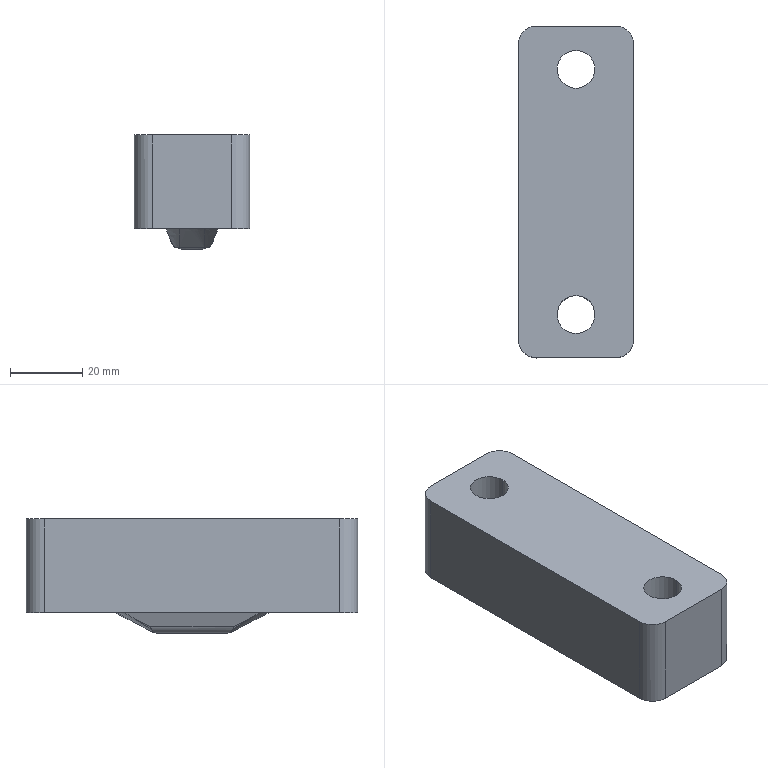Part | STEP file | 1_id690_x_t | 1 solid | 47 faces | box 32 x 92 x 31.644 mm | volume 71708 mm3 | spline 22 | cylinder 14 | plane 11 | commonest cylinder face diameters 10 x4 10.5 x4 15 x4 5.85 x2